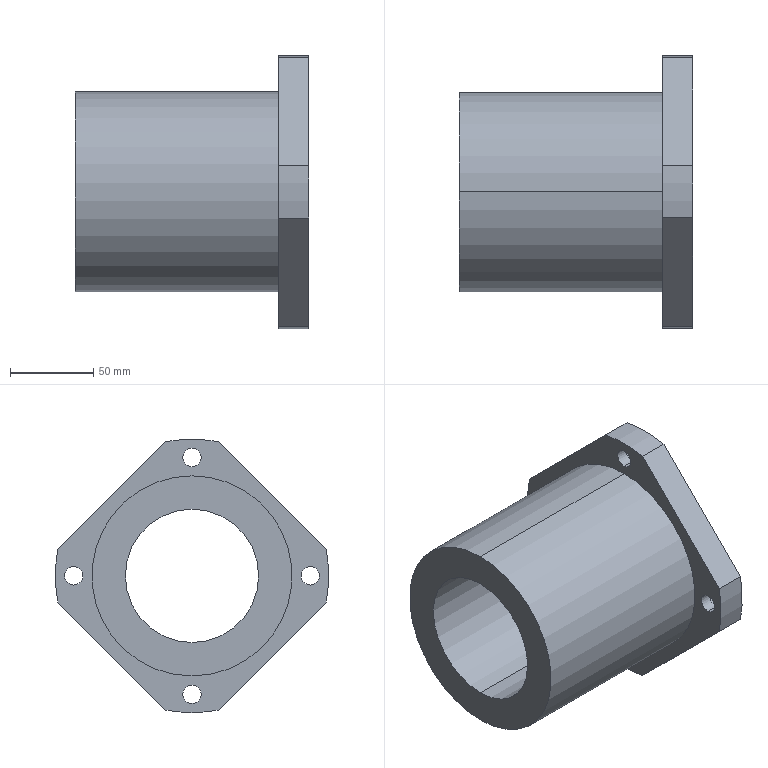Part | STEP file | 001-009-LMK80UU | 1 solid | 36 faces | box 140 x 164 x 164 mm | volume 980879 mm3 | cylinder 25 | plane 11 | commonest cylinder face diameters 11 x8 17 x8 164 x5 80 x2 120 x2